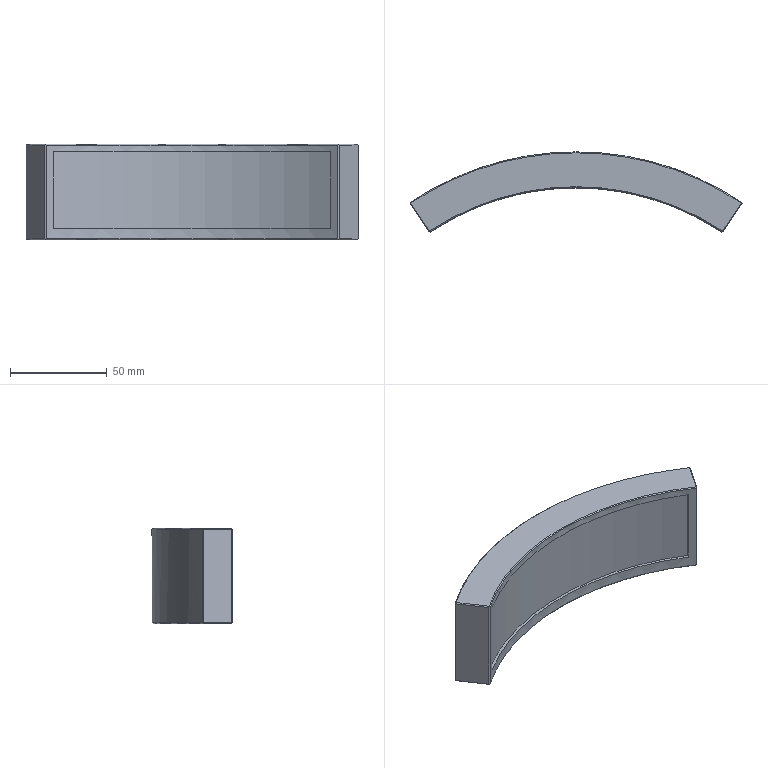Part | SolidWorks | features BaseBody 1 | 1 solid | 47 faces | box 171.672 x 41.389 x 49.5 mm | volume 148043 mm3 | plane 25 | cone 11 | cylinder 11 | commonest cylinder face diameters 2.5 x6 3.5 x2 271 x1 274 x1 308 x1
STEP:
#1=CARTESIAN_POINT('',(-85.424,127.536,49.5));
#2=VERTEX_POINT('',#1);
#3=CARTESIAN_POINT('',(0.,153.501,49.5));
#4=VERTEX_POINT('',#3);
#5=CARTESIAN_POINT('',(0.,0.,49.5));
#6=DIRECTION('',(0.,0.,-1.));
#7=DIRECTION('',(0.,1.,0.));
#8=AXIS2_PLACEMENT_3D('',#5,#6,#7);
#9=CIRCLE('',#8,153.501);
#10=EDGE_CURVE('',#2,#4,#9,.T.);
#11=ORIENTED_EDGE('',*,*,#10,.T.);
#12=CARTESIAN_POINT('',(0.,154.,49.002));
#13=VERTEX_POINT('',#12);
#14=CARTESIAN_POINT('',(0.,154.,49.002));
#15=DIRECTION('',(0.,0.7083,-0.706));
#16=VECTOR('',#15,1000.);
#17=LINE('',#14,#16);
#18=EDGE_CURVE('',#4,#13,#17,.T.);
#19=ORIENTED_EDGE('',*,*,#18,.T.);
#20=CARTESIAN_POINT('',(-85.701,127.95,49.002));
#21=VERTEX_POINT('',#20);
#22=CARTESIAN_POINT('',(0.,0.,49.002));
#23=DIRECTION('',(0.,0.,-1.));
#24=DIRECTION('',(-1.,0.,0.));
#25=AXIS2_PLACEMENT_3D('',#22,#23,#24);
#26=CIRCLE('',#25,154.);
#27=EDGE_CURVE('',#21,#13,#26,.T.);
#28=ORIENTED_EDGE('',*,*,#27,.F.);
#29=CARTESIAN_POINT('',(-85.424,127.536,49.5));
#30=DIRECTION('',(0.3941,-0.5885,0.706));
#31=VECTOR('',#30,1000.);
#32=LINE('',#29,#31);
#33=EDGE_CURVE('',#21,#2,#32,.T.);
#34=ORIENTED_EDGE('',*,*,#33,.T.);
#35=EDGE_LOOP('',(#11,#19,#28,#34));
#36=FACE_OUTER_BOUND('',#35,.T.);
#37=CARTESIAN_POINT('',(0.,0.,49.002));
#38=DIRECTION('',(0.,0.,-1.));
#39=DIRECTION('',(0.,1.,0.));
#40=AXIS2_PLACEMENT_3D('',#37,#38,#39);
#41=CONICAL_SURFACE('',#40,154.,0.787);
#42=ADVANCED_FACE('',(#36),#41,.T.);
#43=CARTESIAN_POINT('',(52.605,139.416,43.5));
#44=VERTEX_POINT('',#43);
#45=CARTESIAN_POINT('',(49.317,140.613,43.5));
#46=VERTEX_POINT('',#45);
#47=CARTESIAN_POINT('',(50.961,140.014,43.5));
#48=DIRECTION('',(0.342,0.9397,0.));
#49=DIRECTION('',(-0.9397,0.342,0.));
#50=AXIS2_PLACEMENT_3D('',#47,#48,#49);
#51=CIRCLE('',#50,1.75);
#52=EDGE_CURVE('',#44,#46,#51,.T.);
#53=ORIENTED_EDGE('',*,*,#52,.F.);
#54=CARTESIAN_POINT('',(54.312,144.105,43.5));
#55=VERTEX_POINT('',#54);
#56=CARTESIAN_POINT('',(54.316,144.114,43.5));
#57=DIRECTION('',(0.342,0.9397,0.));
#58=VECTOR('',#57,1000.);
#59=LINE('',#56,#58);
#60=EDGE_CURVE('',#44,#55,#59,.T.);
#61=ORIENTED_EDGE('',*,*,#60,.T.);
#62=CARTESIAN_POINT('',(51.023,145.302,43.5));
#63=VERTEX_POINT('',#62);
#64=CARTESIAN_POINT('',(51.023,145.302,43.5));
#65=CARTESIAN_POINT('',(51.023,145.302,43.384));
#66=CARTESIAN_POINT('',(51.034,145.298,43.271));
#67=CARTESIAN_POINT('',(51.076,145.283,43.047));
#68=CARTESIAN_POINT('',(51.108,145.272,42.936));
#69=CARTESIAN_POINT('',(51.19,145.243,42.724));
#70=CARTESIAN_POINT('',(51.241,145.225,42.624));
#71=CARTESIAN_POINT('',(51.361,145.183,42.433));
#72=CARTESIAN_POINT('',(51.431,145.158,42.343));
#73=CARTESIAN_POINT('',(51.659,145.077,42.101));
#74=CARTESIAN_POINT('',(51.843,145.012,41.971));
#75=CARTESIAN_POINT('',(52.239,144.869,41.796));
#76=CARTESIAN_POINT('',(52.456,144.791,41.75));
#77=CARTESIAN_POINT('',(52.777,144.674,41.75));
#78=CARTESIAN_POINT('',(52.886,144.634,41.761));
#79=CARTESIAN_POINT('',(53.097,144.557,41.806));
#80=CARTESIAN_POINT('',(53.199,144.519,41.839));
#81=CARTESIAN_POINT('',(53.398,144.446,41.926));
#82=CARTESIAN_POINT('',(53.494,144.41,41.981));
#83=CARTESIAN_POINT('',(53.672,144.344,42.108));
#84=CARTESIAN_POINT('',(53.755,144.314,42.18));
#85=CARTESIAN_POINT('',(53.908,144.257,42.343));
#86=CARTESIAN_POINT('',(53.976,144.231,42.432));
#87=CARTESIAN_POINT('',(54.095,144.187,42.621));
#88=CARTESIAN_POINT('',(54.146,144.167,42.723));
#89=CARTESIAN_POINT('',(54.269,144.121,43.042));
#90=CARTESIAN_POINT('',(54.312,144.105,43.269));
#91=CARTESIAN_POINT('',(54.312,144.105,43.5));
#92=B_SPLINE_CURVE_WITH_KNOTS('',3,(#64,#65,#66,#67,#68,#69,#70,#71,#72,#73,#74,#75,#76,#77,#78,#79,#80,#81,#82,#83,#84,#85,#86,#87,#88,#89,#90,#91),.UNSPECIFIED.,.F.,.F.,(4,2,2,2,2,2,2,2,2,2,2,2,2,4),(0.,0.0003419,0.0006838,0.001026,0.001368,0.002051,0.002735,0.003077,0.003419,0.003761,0.004103,0.004445,0.004786,0.00547),.UNSPECIFIED.);
#93=EDGE_CURVE('',#63,#55,#92,.T.);
#94=ORIENTED_EDGE('',*,*,#93,.F.);
#95=CARTESIAN_POINT('',(51.027,145.311,43.5));
#96=DIRECTION('',(0.342,0.9397,0.));
#97=VECTOR('',#96,1000.);
#98=LINE('',#95,#97);
#99=EDGE_CURVE('',#46,#63,#98,.T.);
#100=ORIENTED_EDGE('',*,*,#99,.F.);
#101=EDGE_LOOP('',(#53,#61,#94,#100));
#102=FACE_OUTER_BOUND('',#101,.T.);
#103=CARTESIAN_POINT('',(52.671,144.713,43.5));
#104=DIRECTION('',(0.342,0.9397,0.));
#105=DIRECTION('',(-0.9397,0.342,0.));
#106=AXIS2_PLACEMENT_3D('',#103,#104,#105);
#107=CYLINDRICAL_SURFACE('',#106,1.75);
#108=ADVANCED_FACE('',(#102),#107,.F.);
#109=CARTESIAN_POINT('',(1.25,143.5,6.));
#110=VERTEX_POINT('',#109);
#111=CARTESIAN_POINT('',(-1.25,143.5,6.));
#112=VERTEX_POINT('',#111);
#113=CARTESIAN_POINT('',(0.,143.5,6.));
#114=DIRECTION('',(0.,0.,-1.));
#115=DIRECTION('',(-1.,0.,0.));
#116=AXIS2_PLACEMENT_3D('',#113,#114,#115);
#117=CIRCLE('',#116,1.25);
#118=EDGE_CURVE('',#110,#112,#117,.T.);
#119=ORIENTED_EDGE('',*,*,#118,.F.);
#120=CARTESIAN_POINT('',(1.25,143.5,0.));
#121=VERTEX_POINT('',#120);
#122=CARTESIAN_POINT('',(1.25,143.5,0.));
#123=DIRECTION('',(0.,0.,-1.));
#124=VECTOR('',#123,1000.);
#125=LINE('',#122,#124);
#126=EDGE_CURVE('',#110,#121,#125,.T.);
#127=ORIENTED_EDGE('',*,*,#126,.T.);
#128=CARTESIAN_POINT('',(-1.25,143.5,0.));
#129=VERTEX_POINT('',#128);
#130=CARTESIAN_POINT('',(0.,143.5,0.));
#131=DIRECTION('',(0.,0.,-1.));
#132=DIRECTION('',(-1.,0.,0.));
#133=AXIS2_PLACEMENT_3D('',#130,#131,#132);
#134=CIRCLE('',#133,1.25);
#135=EDGE_CURVE('',#121,#129,#134,.T.);
#136=ORIENTED_EDGE('',*,*,#135,.T.);
#137=CARTESIAN_POINT('',(-1.25,143.5,0.));
#138=DIRECTION('',(0.,0.,-1.));
#139=VECTOR('',#138,1000.);
#140=LINE('',#137,#139);
#141=EDGE_CURVE('',#112,#129,#140,.T.);
#142=ORIENTED_EDGE('',*,*,#141,.F.);
#143=EDGE_LOOP('',(#119,#127,#136,#142));
#144=FACE_OUTER_BOUND('',#143,.T.);
#145=CARTESIAN_POINT('',(0.,143.5,0.));
#146=DIRECTION('',(0.,0.,-1.));
#147=DIRECTION('',(-1.,0.,0.));
#148=AXIS2_PLACEMENT_3D('',#145,#146,#147);
#149=CYLINDRICAL_SURFACE('',#148,1.25);
#150=ADVANCED_FACE('',(#144),#149,.F.);
#151=CARTESIAN_POINT('',(49.269,135.227,6.));
#152=VERTEX_POINT('',#151);
#153=CARTESIAN_POINT('',(48.019,133.977,6.));
#154=VERTEX_POINT('',#153);
#155=CARTESIAN_POINT('',(48.019,135.227,6.));
#156=DIRECTION('',(0.,0.,-1.));
#157=DIRECTION('',(-1.,0.,0.));
#158=AXIS2_PLACEMENT_3D('',#155,#156,#157);
#159=CIRCLE('',#158,1.25);
#160=EDGE_CURVE('',#152,#154,#159,.T.);
#161=ORIENTED_EDGE('',*,*,#160,.F.);
#162=CARTESIAN_POINT('',(49.269,135.227,0.));
#163=VERTEX_POINT('',#162);
#164=CARTESIAN_POINT('',(49.269,135.227,0.));
#165=DIRECTION('',(0.,0.,-1.));
#166=VECTOR('',#165,1000.);
#167=LINE('',#164,#166);
#168=EDGE_CURVE('',#152,#163,#167,.T.);
#169=ORIENTED_EDGE('',*,*,#168,.T.);
#170=CARTESIAN_POINT('',(46.769,135.227,0.));
#171=VERTEX_POINT('',#170);
#172=CARTESIAN_POINT('',(48.019,135.227,0.));
#173=DIRECTION('',(0.,0.,-1.));
#174=DIRECTION('',(-1.,0.,0.));
#175=AXIS2_PLACEMENT_3D('',#172,#173,#174);
#176=CIRCLE('',#175,1.25);
#177=EDGE_CURVE('',#163,#171,#176,.T.);
#178=ORIENTED_EDGE('',*,*,#177,.T.);
#179=CARTESIAN_POINT('',(46.769,135.227,6.));
#180=VERTEX_POINT('',#179);
#181=CARTESIAN_POINT('',(46.769,135.227,0.));
#182=DIRECTION('',(0.,0.,-1.));
#183=VECTOR('',#182,1000.);
#184=LINE('',#181,#183);
#185=EDGE_CURVE('',#180,#171,#184,.T.);
#186=ORIENTED_EDGE('',*,*,#185,.F.);
#187=CARTESIAN_POINT('',(48.019,135.227,6.));
#188=DIRECTION('',(0.,0.,-1.));
#189=DIRECTION('',(-1.,0.,0.));
#190=AXIS2_PLACEMENT_3D('',#187,#188,#189);
#191=CIRCLE('',#190,1.25);
#192=EDGE_CURVE('',#154,#180,#191,.T.);
#193=ORIENTED_EDGE('',*,*,#192,.F.);
#194=EDGE_LOOP('',(#161,#169,#178,#186,#193));
#195=FACE_OUTER_BOUND('',#194,.T.);
#196=CARTESIAN_POINT('',(48.019,135.227,0.));
#197=DIRECTION('',(0.,0.,-1.));
#198=DIRECTION('',(-1.,0.,0.));
#199=AXIS2_PLACEMENT_3D('',#196,#197,#198);
#200=CYLINDRICAL_SURFACE('',#199,1.25);
#201=ADVANCED_FACE('',(#195),#200,.F.);
#202=CARTESIAN_POINT('',(-46.769,135.227,6.));
#203=VERTEX_POINT('',#202);
#204=CARTESIAN_POINT('',(-49.269,135.227,6.));
#205=VERTEX_POINT('',#204);
#206=CARTESIAN_POINT('',(-48.019,135.227,6.));
#207=DIRECTION('',(0.,0.,-1.));
#208=DIRECTION('',(-1.,0.,0.));
#209=AXIS2_PLACEMENT_3D('',#206,#207,#208);
#210=CIRCLE('',#209,1.25);
#211=EDGE_CURVE('',#203,#205,#210,.T.);
#212=ORIENTED_EDGE('',*,*,#211,.F.);
#213=CARTESIAN_POINT('',(-46.769,135.227,0.));
#214=VERTEX_POINT('',#213);
#215=CARTESIAN_POINT('',(-46.769,135.227,0.));
#216=DIRECTION('',(0.,0.,-1.));
#217=VECTOR('',#216,1000.);
#218=LINE('',#215,#217);
#219=EDGE_CURVE('',#203,#214,#218,.T.);
#220=ORIENTED_EDGE('',*,*,#219,.T.);
#221=CARTESIAN_POINT('',(-49.269,135.227,0.));
#222=VERTEX_POINT('',#221);
#223=CARTESIAN_POINT('',(-48.019,135.227,0.));
#224=DIRECTION('',(0.,0.,-1.));
#225=DIRECTION('',(-1.,0.,0.));
#226=AXIS2_PLACEMENT_3D('',#223,#224,#225);
#227=CIRCLE('',#226,1.25);
#228=EDGE_CURVE('',#214,#222,#227,.T.);
#229=ORIENTED_EDGE('',*,*,#228,.T.);
#230=CARTESIAN_POINT('',(-49.269,135.227,0.));
#231=DIRECTION('',(0.,0.,-1.));
#232=VECTOR('',#231,1000.);
#233=LINE('',#230,#232);
#234=EDGE_CURVE('',#205,#222,#233,.T.);
#235=ORIENTED_EDGE('',*,*,#234,.F.);
#236=EDGE_LOOP('',(#212,#220,#229,#235));
#237=FACE_OUTER_BOUND('',#236,.T.);
#238=CARTESIAN_POINT('',(-48.019,135.227,0.));
#239=DIRECTION('',(0.,0.,-1.));
#240=DIRECTION('',(-1.,0.,0.));
#241=AXIS2_PLACEMENT_3D('',#238,#239,#240);
#242=CYLINDRICAL_SURFACE('',#241,1.25);
#243=ADVANCED_FACE('',(#237),#242,.F.);
#244=CARTESIAN_POINT('',(0.,143.5,6.751));
#245=VERTEX_POINT('',#244);
#246=CARTESIAN_POINT('',(-1.25,143.5,6.));
#247=DIRECTION('',(-0.8572,0.,-0.515));
#248=VECTOR('',#247,1000.);
#249=LINE('',#246,#248);
#250=EDGE_CURVE('',#245,#112,#249,.T.);
#251=ORIENTED_EDGE('',*,*,#250,.F.);
#252=CARTESIAN_POINT('',(1.25,143.5,6.));
#253=DIRECTION('',(0.8572,0.,-0.515));
#254=VECTOR('',#253,1000.);
#255=LINE('',#252,#254);
#256=EDGE_CURVE('',#245,#110,#255,.T.);
#257=ORIENTED_EDGE('',*,*,#256,.T.);
#258=ORIENTED_EDGE('',*,*,#118,.T.);
#259=EDGE_LOOP('',(#251,#257,#258));
#260=FACE_OUTER_BOUND('',#259,.T.);
#261=CARTESIAN_POINT('',(0.,143.5,6.));
#262=DIRECTION('',(0.,0.,-1.));
#263=DIRECTION('',(-1.,0.,0.));
#264=AXIS2_PLACEMENT_3D('',#261,#262,#263);
#265=CONICAL_SURFACE('',#264,1.25,1.03);
#266=ADVANCED_FACE('',(#260),#265,.F.);
#267=CARTESIAN_POINT('',(48.019,135.227,6.751));
#268=VERTEX_POINT('',#267);
#269=CARTESIAN_POINT('',(48.019,136.477,6.));
#270=VERTEX_POINT('',#269);
#271=CARTESIAN_POINT('',(48.019,136.477,6.));
#272=DIRECTION('',(0.,0.8572,-0.515));
#273=VECTOR('',#272,1000.);
#274=LINE('',#271,#273);
#275=EDGE_CURVE('',#268,#270,#274,.T.);
#276=ORIENTED_EDGE('',*,*,#275,.F.);
#277=CARTESIAN_POINT('',(48.019,133.977,6.));
#278=DIRECTION('',(0.,-0.8572,-0.515));
#279=VECTOR('',#278,1000.);
#280=LINE('',#277,#279);
#281=EDGE_CURVE('',#268,#154,#280,.T.);
#282=ORIENTED_EDGE('',*,*,#281,.T.);
#283=ORIENTED_EDGE('',*,*,#192,.T.);
#284=CARTESIAN_POINT('',(48.019,135.227,6.));
#285=DIRECTION('',(0.,0.,-1.));
#286=DIRECTION('',(-1.,0.,0.));
#287=AXIS2_PLACEMENT_3D('',#284,#285,#286);
#288=CIRCLE('',#287,1.25);
#289=EDGE_CURVE('',#180,#270,#288,.T.);
#290=ORIENTED_EDGE('',*,*,#289,.T.);
#291=EDGE_LOOP('',(#276,#282,#283,#290));
#292=FACE_OUTER_BOUND('',#291,.T.);
#293=CARTESIAN_POINT('',(48.019,135.227,6.));
#294=DIRECTION('',(0.,0.,-1.));
#295=DIRECTION('',(0.,1.,0.));
#296=AXIS2_PLACEMENT_3D('',#293,#294,#295);
#297=CONICAL_SURFACE('',#296,1.25,1.03);
#298=ADVANCED_FACE('',(#292),#297,.F.);
#299=CARTESIAN_POINT('',(-48.019,135.227,6.751));
#300=VERTEX_POINT('',#299);
#301=CARTESIAN_POINT('',(-49.269,135.227,6.));
#302=DIRECTION('',(-0.8572,0.,-0.515));
#303=VECTOR('',#302,1000.);
#304=LINE('',#301,#303);
#305=EDGE_CURVE('',#300,#205,#304,.T.);
#306=ORIENTED_EDGE('',*,*,#305,.F.);
#307=CARTESIAN_POINT('',(-46.769,135.227,6.));
#308=DIRECTION('',(0.8572,0.,-0.515));
#309=VECTOR('',#308,1000.);
#310=LINE('',#307,#309);
#311=EDGE_CURVE('',#300,#203,#310,.T.);
#312=ORIENTED_EDGE('',*,*,#311,.T.);
#313=ORIENTED_EDGE('',*,*,#211,.T.);
#314=EDGE_LOOP('',(#306,#312,#313));
#315=FACE_OUTER_BOUND('',#314,.T.);
#316=CARTESIAN_POINT('',(-48.019,135.227,6.));
#317=DIRECTION('',(0.,0.,-1.));
#318=DIRECTION('',(-1.,0.,0.));
#319=AXIS2_PLACEMENT_3D('',#316,#317,#318);
#320=CONICAL_SURFACE('',#319,1.25,1.03);
#321=ADVANCED_FACE('',(#315),#320,.F.);
#322=ORIENTED_EDGE('',*,*,#27,.T.);
#323=CARTESIAN_POINT('',(85.701,127.95,49.002));
#324=VERTEX_POINT('',#323);
#325=CARTESIAN_POINT('',(0.,0.,49.002));
#326=DIRECTION('',(0.,0.,-1.));
#327=DIRECTION('',(-1.,0.,0.));
#328=AXIS2_PLACEMENT_3D('',#325,#326,#327);
#329=CIRCLE('',#328,154.);
#330=EDGE_CURVE('',#13,#324,#329,.T.);
#331=ORIENTED_EDGE('',*,*,#330,.T.);
#332=CARTESIAN_POINT('',(85.701,127.95,0.4976));
#333=VERTEX_POINT('',#332);
#334=CARTESIAN_POINT('',(85.701,127.95,49.5));
#335=DIRECTION('',(0.,0.,-1.));
#336=VECTOR('',#335,1000.);
#337=LINE('',#334,#336);
#338=EDGE_CURVE('',#324,#333,#337,.T.);
#339=ORIENTED_EDGE('',*,*,#338,.T.);
#340=CARTESIAN_POINT('',(-85.701,127.95,0.4976));
#341=VERTEX_POINT('',#340);
#342=CARTESIAN_POINT('',(0.,0.,0.4976));
#343=DIRECTION('',(0.,0.,1.));
#344=DIRECTION('',(-1.,0.,0.));
#345=AXIS2_PLACEMENT_3D('',#342,#343,#344);
#346=CIRCLE('',#345,154.);
#347=EDGE_CURVE('',#333,#341,#346,.T.);
#348=ORIENTED_EDGE('',*,*,#347,.T.);
#349=CARTESIAN_POINT('',(-85.701,127.95,49.5));
#350=DIRECTION('',(0.,0.,1.));
#351=VECTOR('',#350,1000.);
#352=LINE('',#349,#351);
#353=EDGE_CURVE('',#341,#21,#352,.T.);
#354=ORIENTED_EDGE('',*,*,#353,.T.);
#355=EDGE_LOOP('',(#322,#331,#339,#348,#354));
#356=FACE_OUTER_BOUND('',#355,.T.);
#357=ORIENTED_EDGE('',*,*,#93,.T.);
#358=CARTESIAN_POINT('',(54.312,144.105,43.5));
#359=CARTESIAN_POINT('',(54.312,144.105,43.616));
#360=CARTESIAN_POINT('',(54.302,144.109,43.729));
#361=CARTESIAN_POINT('',(54.26,144.124,43.953));
#362=CARTESIAN_POINT('',(54.228,144.136,44.064));
#363=CARTESIAN_POINT('',(54.146,144.167,44.276));
#364=CARTESIAN_POINT('',(54.096,144.186,44.376));
#365=CARTESIAN_POINT('',(53.977,144.231,44.567));
#366=CARTESIAN_POINT('',(53.908,144.257,44.657));
#367=CARTESIAN_POINT('',(53.681,144.341,44.899));
#368=CARTESIAN_POINT('',(53.498,144.409,45.029));
#369=CARTESIAN_POINT('',(53.103,144.555,45.204));
#370=CARTESIAN_POINT('',(52.887,144.634,45.25));
#371=CARTESIAN_POINT('',(52.565,144.751,45.25));
#372=CARTESIAN_POINT('',(52.456,144.791,45.239));
#373=CARTESIAN_POINT('',(52.245,144.867,45.194));
#374=CARTESIAN_POINT('',(52.142,144.904,45.161));
#375=CARTESIAN_POINT('',(51.943,144.976,45.074));
#376=CARTESIAN_POINT('',(51.846,145.01,45.019));
#377=CARTESIAN_POINT('',(51.668,145.074,44.892));
#378=CARTESIAN_POINT('',(51.584,145.104,44.82));
#379=CARTESIAN_POINT('',(51.43,145.158,44.657));
#380=CARTESIAN_POINT('',(51.362,145.182,44.568));
#381=CARTESIAN_POINT('',(51.242,145.225,44.379));
#382=CARTESIAN_POINT('',(51.191,145.243,44.277));
#383=CARTESIAN_POINT('',(51.066,145.287,43.958));
#384=CARTESIAN_POINT('',(51.023,145.302,43.731));
#385=CARTESIAN_POINT('',(51.023,145.302,43.5));
#386=B_SPLINE_CURVE_WITH_KNOTS('',3,(#358,#359,#360,#361,#362,#363,#364,#365,#366,#367,#368,#369,#370,#371,#372,#373,#374,#375,#376,#377,#378,#379,#380,#381,#382,#383,#384,#385),.UNSPECIFIED.,.F.,.F.,(4,2,2,2,2,2,2,2,2,2,2,2,2,4),(0.00547,0.005812,0.006154,0.006496,0.006838,0.007522,0.008205,0.008547,0.008889,0.009231,0.009573,0.009915,0.01026,0.01094),.UNSPECIFIED.);
#387=EDGE_CURVE('',#55,#63,#386,.T.);
#388=ORIENTED_EDGE('',*,*,#387,.T.);
#389=EDGE_LOOP('',(#357,#388));
#390=FACE_BOUND('',#389,.T.);
#391=CARTESIAN_POINT('',(0.,0.,49.5));
#392=DIRECTION('',(0.,0.,-1.));
#393=DIRECTION('',(-1.,0.,0.));
#394=AXIS2_PLACEMENT_3D('',#391,#392,#393);
#395=CYLINDRICAL_SURFACE('',#394,154.);
#396=ADVANCED_FACE('',(#356,#390),#395,.T.);
#397=ORIENTED_EDGE('',*,*,#338,.F.);
#398=CARTESIAN_POINT('',(85.836,127.257,49.001));
#399=VERTEX_POINT('',#398);
#400=CARTESIAN_POINT('',(85.836,127.257,49.001));
#401=DIRECTION('',(-0.1908,0.9816,0.002296));
#402=VECTOR('',#401,1000.);
#403=LINE('',#400,#402);
#404=EDGE_CURVE('',#399,#324,#403,.T.);
#405=ORIENTED_EDGE('',*,*,#404,.F.);
#406=CARTESIAN_POINT('',(85.836,127.257,0.4992));
#407=VERTEX_POINT('',#406);
#408=CARTESIAN_POINT('',(85.836,127.257,49.5));
#409=DIRECTION('',(0.,0.,1.));
#410=VECTOR('',#409,1000.);
#411=LINE('',#408,#410);
#412=EDGE_CURVE('',#407,#399,#411,.T.);
#413=ORIENTED_EDGE('',*,*,#412,.F.);
#414=CARTESIAN_POINT('',(85.701,127.95,0.4976));
#415=DIRECTION('',(0.1908,-0.9816,0.002296));
#416=VECTOR('',#415,1000.);
#417=LINE('',#414,#416);
#418=EDGE_CURVE('',#333,#407,#417,.T.);
#419=ORIENTED_EDGE('',*,*,#418,.F.);
#420=EDGE_LOOP('',(#397,#405,#413,#419));
#421=FACE_OUTER_BOUND('',#420,.T.);
#422=CARTESIAN_POINT('',(85.701,127.95,49.5));
#423=DIRECTION('',(-0.9816,-0.1908,0.));
#424=DIRECTION('',(0.1908,-0.9816,0.));
#425=AXIS2_PLACEMENT_3D('',#422,#423,#424);
#426=PLANE('',#425);
#427=ADVANCED_FACE('',(#421),#426,.F.);
#428=ORIENTED_EDGE('',*,*,#18,.F.);
#429=CARTESIAN_POINT('',(85.424,127.536,49.5));
#430=VERTEX_POINT('',#429);
#431=CARTESIAN_POINT('',(0.,0.,49.5));
#432=DIRECTION('',(0.,0.,-1.));
#433=DIRECTION('',(0.,1.,0.));
#434=AXIS2_PLACEMENT_3D('',#431,#432,#433);
#435=CIRCLE('',#434,153.501);
#436=EDGE_CURVE('',#4,#430,#435,.T.);
#437=ORIENTED_EDGE('',*,*,#436,.T.);
#438=CARTESIAN_POINT('',(85.424,127.536,49.5));
#439=DIRECTION('',(0.3941,0.5885,-0.706));
#440=VECTOR('',#439,1000.);
#441=LINE('',#438,#440);
#442=EDGE_CURVE('',#430,#324,#441,.T.);
#443=ORIENTED_EDGE('',*,*,#442,.T.);
#444=ORIENTED_EDGE('',*,*,#330,.F.);
#445=EDGE_LOOP('',(#428,#437,#443,#444));
#446=FACE_OUTER_BOUND('',#445,.T.);
#447=CARTESIAN_POINT('',(0.,0.,49.002));
#448=DIRECTION('',(0.,0.,-1.));
#449=DIRECTION('',(0.,1.,0.));
#450=AXIS2_PLACEMENT_3D('',#447,#448,#449);
#451=CONICAL_SURFACE('',#450,154.,0.787);
#452=ADVANCED_FACE('',(#446),#451,.T.);
#453=CARTESIAN_POINT('',(-85.836,127.257,49.001));
#454=VERTEX_POINT('',#453);
#455=CARTESIAN_POINT('',(-85.836,127.257,0.4976));
#456=VERTEX_POINT('',#455);
#457=CARTESIAN_POINT('',(-85.836,127.257,49.5));
#458=DIRECTION('',(0.,0.,-1.));
#459=VECTOR('',#458,1000.);
#460=LINE('',#457,#459);
#461=EDGE_CURVE('',#454,#456,#460,.T.);
#462=ORIENTED_EDGE('',*,*,#461,.F.);
#463=CARTESIAN_POINT('',(-85.701,127.95,49.002));
#464=DIRECTION('',(-0.1908,-0.9816,-0.002296));
#465=VECTOR('',#464,1000.);
#466=LINE('',#463,#465);
#467=EDGE_CURVE('',#21,#454,#466,.T.);
#468=ORIENTED_EDGE('',*,*,#467,.F.);
#469=ORIENTED_EDGE('',*,*,#353,.F.);
#470=CARTESIAN_POINT('',(-85.836,127.257,0.4976));
#471=DIRECTION('',(0.1908,0.9816,0.));
#472=VECTOR('',#471,1000.);
#473=LINE('',#470,#472);
#474=EDGE_CURVE('',#456,#341,#473,.T.);
#475=ORIENTED_EDGE('',*,*,#474,.F.);
#476=EDGE_LOOP('',(#462,#468,#469,#475));
#477=FACE_OUTER_BOUND('',#476,.T.);
#478=CARTESIAN_POINT('',(-85.836,127.257,49.5));
#479=DIRECTION('',(0.9816,-0.1908,0.));
#480=DIRECTION('',(0.1908,0.9816,0.));
#481=AXIS2_PLACEMENT_3D('',#478,#479,#480);
#482=PLANE('',#481);
#483=ADVANCED_FACE('',(#477),#482,.F.);
#484=CARTESIAN_POINT('',(-85.422,127.536,0.));
#485=VERTEX_POINT('',#484);
#486=CARTESIAN_POINT('',(-85.422,127.536,0.));
#487=CARTESIAN_POINT('',(-85.515,127.674,0.1659));
#488=CARTESIAN_POINT('',(-85.608,127.812,0.3317));
#489=CARTESIAN_POINT('',(-85.701,127.95,0.4976));
#490=B_SPLINE_CURVE_WITH_KNOTS('',3,(#486,#487,#488,#489),.UNSPECIFIED.,.F.,.F.,(4,4),(0.,1.),.UNSPECIFIED.);
#491=EDGE_CURVE('',#485,#341,#490,.T.);
#492=ORIENTED_EDGE('',*,*,#491,.T.);
#493=ORIENTED_EDGE('',*,*,#347,.F.);
#494=CARTESIAN_POINT('',(85.424,127.536,0.));
#495=VERTEX_POINT('',#494);
#496=CARTESIAN_POINT('',(85.701,127.95,0.4976));
#497=DIRECTION('',(-0.3941,-0.5885,-0.706));
#498=VECTOR('',#497,1000.);
#499=LINE('',#496,#498);
#500=EDGE_CURVE('',#333,#495,#499,.T.);
#501=ORIENTED_EDGE('',*,*,#500,.T.);
#502=CARTESIAN_POINT('',(0.,0.,0.));
#503=DIRECTION('',(0.,0.,1.));
#504=DIRECTION('',(1.,0.,0.));
#505=AXIS2_PLACEMENT_3D('',#502,#503,#504);
#506=CIRCLE('',#505,153.501);
#507=EDGE_CURVE('',#495,#485,#506,.T.);
#508=ORIENTED_EDGE('',*,*,#507,.T.);
#509=EDGE_LOOP('',(#492,#493,#501,#508));
#510=FACE_OUTER_BOUND('',#509,.T.);
#511=CARTESIAN_POINT('',(0.,0.,0.4976));
#512=DIRECTION('',(0.,0.,1.));
#513=DIRECTION('',(1.,0.,0.));
#514=AXIS2_PLACEMENT_3D('',#511,#512,#513);
#515=CONICAL_SURFACE('',#514,154.,0.787);
#516=ADVANCED_FACE('',(#510),#515,.T.);
#517=ORIENTED_EDGE('',*,*,#60,.F.);
#518=CARTESIAN_POINT('',(50.961,140.014,43.5));
#519=DIRECTION('',(0.342,0.9397,0.));
#520=DIRECTION('',(-0.9397,0.342,0.));
#521=AXIS2_PLACEMENT_3D('',#518,#519,#520);
#522=CIRCLE('',#521,1.75);
#523=EDGE_CURVE('',#46,#44,#522,.T.);
#524=ORIENTED_EDGE('',*,*,#523,.F.);
#525=ORIENTED_EDGE('',*,*,#99,.T.);
#526=ORIENTED_EDGE('',*,*,#387,.F.);
#527=EDGE_LOOP('',(#517,#524,#525,#526));
#528=FACE_OUTER_BOUND('',#527,.T.);
#529=CARTESIAN_POINT('',(52.671,144.713,43.5));
#530=DIRECTION('',(0.342,0.9397,0.));
#531=DIRECTION('',(-0.9397,0.342,0.));
#532=AXIS2_PLACEMENT_3D('',#529,#530,#531);
#533=CYLINDRICAL_SURFACE('',#532,1.75);
#534=ADVANCED_FACE('',(#528),#533,.F.);
#535=CARTESIAN_POINT('',(85.836,127.257,0.4992));
#536=DIRECTION('',(-0.5853,0.3948,-0.7083));
#537=VECTOR('',#536,1000.);
#538=LINE('',#535,#537);
#539=EDGE_CURVE('',#407,#495,#538,.T.);
#540=ORIENTED_EDGE('',*,*,#539,.T.);
#541=ORIENTED_EDGE('',*,*,#500,.F.);
#542=ORIENTED_EDGE('',*,*,#418,.T.);
#543=EDGE_LOOP('',(#540,#541,#542));
#544=FACE_OUTER_BOUND('',#543,.T.);
#545=CARTESIAN_POINT('',(85.424,127.536,0.));
#546=DIRECTION('',(0.8022,0.1546,-0.5767));
#547=DIRECTION('',(-0.5837,0.,-0.8119));
#548=AXIS2_PLACEMENT_3D('',#545,#546,#547);
#549=PLANE('',#548);
#550=ADVANCED_FACE('',(#544),#549,.T.);
#551=ORIENTED_EDGE('',*,*,#404,.T.);
#552=ORIENTED_EDGE('',*,*,#442,.F.);
#553=CARTESIAN_POINT('',(85.836,127.257,49.001));
#554=DIRECTION('',(-0.5853,0.3948,0.7083));
#555=VECTOR('',#554,1000.);
#556=LINE('',#553,#555);
#557=EDGE_CURVE('',#399,#430,#556,.T.);
#558=ORIENTED_EDGE('',*,*,#557,.F.);
#559=EDGE_LOOP('',(#551,#552,#558));
#560=FACE_OUTER_BOUND('',#559,.T.);
#561=CARTESIAN_POINT('',(85.424,127.536,49.5));
#562=DIRECTION('',(0.8022,0.1546,0.5767));
#563=DIRECTION('',(0.5837,0.,-0.8119));
#564=AXIS2_PLACEMENT_3D('',#561,#562,#563);
#565=PLANE('',#564);
#566=ADVANCED_FACE('',(#560),#565,.T.);
#567=CARTESIAN_POINT('',(76.049,112.748,0.4992));
#568=VERTEX_POINT('',#567);
#569=CARTESIAN_POINT('',(76.049,112.748,49.001));
#570=VERTEX_POINT('',#569);
#571=CARTESIAN_POINT('',(76.049,112.748,49.5));
#572=DIRECTION('',(0.,0.,1.));
#573=VECTOR('',#572,1000.);
#574=LINE('',#571,#573);
#575=EDGE_CURVE('',#568,#570,#574,.T.);
#576=ORIENTED_EDGE('',*,*,#575,.F.);
#577=CARTESIAN_POINT('',(75.771,112.335,0.4992));
#578=DIRECTION('',(-0.5592,-0.829,0.));
#579=VECTOR('',#578,1000.);
#580=LINE('',#577,#579);
#581=EDGE_CURVE('',#407,#568,#580,.T.);
#582=ORIENTED_EDGE('',*,*,#581,.F.);
#583=ORIENTED_EDGE('',*,*,#412,.T.);
#584=CARTESIAN_POINT('',(75.771,112.335,49.001));
#585=DIRECTION('',(0.5592,0.829,0.));
#586=VECTOR('',#585,1000.);
#587=LINE('',#584,#586);
#588=EDGE_CURVE('',#570,#399,#587,.T.);
#589=ORIENTED_EDGE('',*,*,#588,.F.);
#590=EDGE_LOOP('',(#576,#582,#583,#589));
#591=FACE_OUTER_BOUND('',#590,.T.);
#592=CARTESIAN_POINT('',(75.771,112.335,49.5));
#593=DIRECTION('',(-0.829,0.5592,0.));
#594=DIRECTION('',(-0.5592,-0.829,0.));
#595=AXIS2_PLACEMENT_3D('',#592,#593,#594);
#596=PLANE('',#595);
#597=ADVANCED_FACE('',(#591),#596,.F.);
#598=CARTESIAN_POINT('',(-75.636,113.025,49.5));
#599=VERTEX_POINT('',#598);
#600=CARTESIAN_POINT('',(75.636,113.025,49.5));
#601=VERTEX_POINT('',#600);
#602=CARTESIAN_POINT('',(0.,0.,49.5));
#603=DIRECTION('',(0.,0.,-1.));
#604=DIRECTION('',(0.,-1.,0.));
#605=AXIS2_PLACEMENT_3D('',#602,#603,#604);
#606=CIRCLE('',#605,135.998);
#607=EDGE_CURVE('',#599,#601,#606,.T.);
#608=ORIENTED_EDGE('',*,*,#607,.T.);
#609=CARTESIAN_POINT('',(75.636,113.025,49.5));
#610=DIRECTION('',(0.5592,0.829,0.));
#611=VECTOR('',#610,1000.);
#612=LINE('',#609,#611);
#613=EDGE_CURVE('',#601,#430,#612,.T.);
#614=ORIENTED_EDGE('',*,*,#613,.T.);
#615=ORIENTED_EDGE('',*,*,#436,.F.);
#616=ORIENTED_EDGE('',*,*,#10,.F.);
#617=CARTESIAN_POINT('',(-85.424,127.536,49.5));
#618=DIRECTION('',(0.5592,-0.829,0.));
#619=VECTOR('',#618,1000.);
#620=LINE('',#617,#619);
#621=EDGE_CURVE('',#2,#599,#620,.T.);
#622=ORIENTED_EDGE('',*,*,#621,.T.);
#623=EDGE_LOOP('',(#608,#614,#615,#616,#622));
#624=FACE_OUTER_BOUND('',#623,.T.);
#625=CARTESIAN_POINT('',(0.,0.,49.5));
#626=DIRECTION('',(0.,0.,1.));
#627=DIRECTION('',(1.,0.,0.));
#628=AXIS2_PLACEMENT_3D('',#625,#626,#627);
#629=PLANE('',#628);
#630=ADVANCED_FACE('',(#624),#629,.T.);
#631=ORIENTED_EDGE('',*,*,#467,.T.);
#632=CARTESIAN_POINT('',(-85.836,127.257,49.001));
#633=DIRECTION('',(0.5853,0.3948,0.7083));
#634=VECTOR('',#633,1000.);
#635=LINE('',#632,#634);
#636=EDGE_CURVE('',#454,#2,#635,.T.);
#637=ORIENTED_EDGE('',*,*,#636,.T.);
#638=ORIENTED_EDGE('',*,*,#33,.F.);
#639=EDGE_LOOP('',(#631,#637,#638));
#640=FACE_OUTER_BOUND('',#639,.T.);
#641=CARTESIAN_POINT('',(-85.836,127.257,49.001));
#642=DIRECTION('',(-0.8022,0.1546,0.5767));
#643=DIRECTION('',(0.5837,0.,0.8119));
#644=AXIS2_PLACEMENT_3D('',#641,#642,#643);
#645=PLANE('',#644);
#646=ADVANCED_FACE('',(#640),#645,.T.);
#647=CARTESIAN_POINT('',(-85.422,127.536,0.));
#648=DIRECTION('',(-0.5872,-0.396,0.706));
#649=VECTOR('',#648,1000.);
#650=LINE('',#647,#649);
#651=EDGE_CURVE('',#485,#456,#650,.T.);
#652=ORIENTED_EDGE('',*,*,#651,.T.);
#653=ORIENTED_EDGE('',*,*,#474,.T.);
#654=ORIENTED_EDGE('',*,*,#491,.F.);
#655=EDGE_LOOP('',(#652,#653,#654));
#656=FACE_OUTER_BOUND('',#655,.T.);
#657=CARTESIAN_POINT('',(-85.836,127.257,0.4976));
#658=DIRECTION('',(-0.8006,0.1556,-0.5786));
#659=DIRECTION('',(-0.5857,0.,0.8105));
#660=AXIS2_PLACEMENT_3D('',#657,#658,#659);
#661=PLANE('',#660);
#662=ADVANCED_FACE('',(#656),#661,.T.);
#663=CARTESIAN_POINT('',(-76.049,112.748,49.001));
#664=VERTEX_POINT('',#663);
#665=CARTESIAN_POINT('',(-75.771,112.335,49.001));
#666=DIRECTION('',(0.5592,-0.829,0.));
#667=VECTOR('',#666,1000.);
#668=LINE('',#665,#667);
#669=EDGE_CURVE('',#454,#664,#668,.T.);
#670=ORIENTED_EDGE('',*,*,#669,.F.);
#671=ORIENTED_EDGE('',*,*,#461,.T.);
#672=CARTESIAN_POINT('',(-76.049,112.748,0.4976));
#673=VERTEX_POINT('',#672);
#674=CARTESIAN_POINT('',(-75.771,112.335,0.4976));
#675=DIRECTION('',(-0.5592,0.829,0.));
#676=VECTOR('',#675,1000.);
#677=LINE('',#674,#676);
#678=EDGE_CURVE('',#673,#456,#677,.T.);
#679=ORIENTED_EDGE('',*,*,#678,.F.);
#680=CARTESIAN_POINT('',(-76.049,112.748,49.5));
#681=DIRECTION('',(0.,0.,-1.));
#682=VECTOR('',#681,1000.);
#683=LINE('',#680,#682);
#684=EDGE_CURVE('',#664,#673,#683,.T.);
#685=ORIENTED_EDGE('',*,*,#684,.F.);
#686=EDGE_LOOP('',(#670,#671,#679,#685));
#687=FACE_OUTER_BOUND('',#686,.T.);
#688=CARTESIAN_POINT('',(-75.771,112.335,49.5));
#689=DIRECTION('',(0.829,0.5592,0.));
#690=DIRECTION('',(-0.5592,0.829,0.));
#691=AXIS2_PLACEMENT_3D('',#688,#689,#690);
#692=PLANE('',#691);
#693=ADVANCED_FACE('',(#687),#692,.F.);
#694=CARTESIAN_POINT('',(0.,143.5,0.));
#695=DIRECTION('',(0.,0.,-1.));
#696=DIRECTION('',(-1.,0.,0.));
#697=AXIS2_PLACEMENT_3D('',#694,#695,#696);
#698=CIRCLE('',#697,1.25);
#699=EDGE_CURVE('',#129,#121,#698,.T.);
#700=ORIENTED_EDGE('',*,*,#699,.F.);
#701=ORIENTED_EDGE('',*,*,#135,.F.);
#702=EDGE_LOOP('',(#700,#701));
#703=FACE_BOUND('',#702,.T.);
#704=CARTESIAN_POINT('',(48.019,135.227,0.));
#705=DIRECTION('',(0.,0.,-1.));
#706=DIRECTION('',(-1.,0.,0.));
#707=AXIS2_PLACEMENT_3D('',#704,#705,#706);
#708=CIRCLE('',#707,1.25);
#709=EDGE_CURVE('',#171,#163,#708,.T.);
#710=ORIENTED_EDGE('',*,*,#709,.F.);
#711=ORIENTED_EDGE('',*,*,#177,.F.);
#712=EDGE_LOOP('',(#710,#711));
#713=FACE_BOUND('',#712,.T.);
#714=CARTESIAN_POINT('',(-48.019,135.227,0.));
#715=DIRECTION('',(0.,0.,-1.));
#716=DIRECTION('',(-1.,0.,0.));
#717=AXIS2_PLACEMENT_3D('',#714,#715,#716);
#718=CIRCLE('',#717,1.25);
#719=EDGE_CURVE('',#222,#214,#718,.T.);
#720=ORIENTED_EDGE('',*,*,#719,.F.);
#721=ORIENTED_EDGE('',*,*,#228,.F.);
#722=EDGE_LOOP('',(#720,#721));
#723=FACE_BOUND('',#722,.T.);
#724=CARTESIAN_POINT('',(-75.635,113.027,0.));
#725=VERTEX_POINT('',#724);
#726=CARTESIAN_POINT('',(-85.422,127.536,0.));
#727=DIRECTION('',(0.5592,-0.829,0.));
#728=VECTOR('',#727,1000.);
#729=LINE('',#726,#728);
#730=EDGE_CURVE('',#485,#725,#729,.T.);
#731=ORIENTED_EDGE('',*,*,#730,.F.);
#732=ORIENTED_EDGE('',*,*,#507,.F.);
#733=CARTESIAN_POINT('',(75.637,113.026,0.));
#734=VERTEX_POINT('',#733);
#735=CARTESIAN_POINT('',(75.637,113.026,0.));
#736=DIRECTION('',(0.5592,0.829,0.));
#737=VECTOR('',#736,1000.);
#738=LINE('',#735,#737);
#739=EDGE_CURVE('',#734,#495,#738,.T.);
#740=ORIENTED_EDGE('',*,*,#739,.F.);
#741=CARTESIAN_POINT('',(0.,0.,0.));
#742=DIRECTION('',(0.,0.,-1.));
#743=DIRECTION('',(-1.,0.,0.));
#744=AXIS2_PLACEMENT_3D('',#741,#742,#743);
#745=CIRCLE('',#744,135.999);
#746=EDGE_CURVE('',#725,#734,#745,.T.);
#747=ORIENTED_EDGE('',*,*,#746,.F.);
#748=EDGE_LOOP('',(#731,#732,#740,#747));
#749=FACE_OUTER_BOUND('',#748,.T.);
#750=CARTESIAN_POINT('',(0.,0.,0.));
#751=DIRECTION('',(0.,0.,1.));
#752=DIRECTION('',(1.,0.,0.));
#753=AXIS2_PLACEMENT_3D('',#750,#751,#752);
#754=PLANE('',#753);
#755=ADVANCED_FACE('',(#703,#713,#723,#749),#754,.F.);
#756=ORIENTED_EDGE('',*,*,#523,.T.);
#757=ORIENTED_EDGE('',*,*,#52,.T.);
#758=EDGE_LOOP('',(#756,#757));
#759=FACE_OUTER_BOUND('',#758,.T.);
#760=CARTESIAN_POINT('',(50.961,140.014,43.5));
#761=DIRECTION('',(-0.342,-0.9397,0.));
#762=DIRECTION('',(0.9397,-0.342,0.));
#763=AXIS2_PLACEMENT_3D('',#760,#761,#762);
#764=PLANE('',#763);
#765=ADVANCED_FACE('',(#759),#764,.F.);
#766=ORIENTED_EDGE('',*,*,#557,.T.);
#767=ORIENTED_EDGE('',*,*,#613,.F.);
#768=CARTESIAN_POINT('',(75.636,113.025,49.5));
#769=DIRECTION('',(0.5865,-0.3929,-0.7083));
#770=VECTOR('',#769,1000.);
#771=LINE('',#768,#770);
#772=EDGE_CURVE('',#601,#570,#771,.T.);
#773=ORIENTED_EDGE('',*,*,#772,.T.);
#774=ORIENTED_EDGE('',*,*,#588,.T.);
#775=EDGE_LOOP('',(#766,#767,#773,#774));
#776=FACE_OUTER_BOUND('',#775,.T.);
#777=CARTESIAN_POINT('',(-0.4125,0.2782,49.5));
#778=DIRECTION('',(0.5872,-0.3961,0.706));
#779=DIRECTION('',(0.7688,0.,-0.6395));
#780=AXIS2_PLACEMENT_3D('',#777,#778,#779);
#781=PLANE('',#780);
#782=ADVANCED_FACE('',(#776),#781,.T.);
#783=ORIENTED_EDGE('',*,*,#575,.T.);
#784=CARTESIAN_POINT('',(75.359,112.611,49.001));
#785=VERTEX_POINT('',#784);
#786=CARTESIAN_POINT('',(76.049,112.748,49.001));
#787=DIRECTION('',(0.981,0.1942,0.));
#788=VECTOR('',#787,1000.);
#789=LINE('',#786,#788);
#790=EDGE_CURVE('',#785,#570,#789,.T.);
#791=ORIENTED_EDGE('',*,*,#790,.F.);
#792=CARTESIAN_POINT('',(75.359,112.611,0.4976));
#793=VERTEX_POINT('',#792);
#794=CARTESIAN_POINT('',(75.359,112.611,49.5));
#795=DIRECTION('',(0.,0.,1.));
#796=VECTOR('',#795,1000.);
#797=LINE('',#794,#796);
#798=EDGE_CURVE('',#793,#785,#797,.T.);
#799=ORIENTED_EDGE('',*,*,#798,.F.);
#800=CARTESIAN_POINT('',(76.049,112.748,0.4992));
#801=DIRECTION('',(-0.981,-0.1942,-0.002304));
#802=VECTOR('',#801,1000.);
#803=LINE('',#800,#802);
#804=EDGE_CURVE('',#568,#793,#803,.T.);
#805=ORIENTED_EDGE('',*,*,#804,.F.);
#806=EDGE_LOOP('',(#783,#791,#799,#805));
#807=FACE_OUTER_BOUND('',#806,.T.);
#808=CARTESIAN_POINT('',(76.049,112.748,49.5));
#809=DIRECTION('',(-0.1942,0.981,0.));
#810=DIRECTION('',(-0.981,-0.1942,0.));
#811=AXIS2_PLACEMENT_3D('',#808,#809,#810);
#812=PLANE('',#811);
#813=ADVANCED_FACE('',(#807),#812,.F.);
#814=ORIENTED_EDGE('',*,*,#581,.T.);
#815=CARTESIAN_POINT('',(75.637,113.026,0.));
#816=DIRECTION('',(0.5853,-0.3948,0.7083));
#817=VECTOR('',#816,1000.);
#818=LINE('',#815,#817);
#819=EDGE_CURVE('',#734,#568,#818,.T.);
#820=ORIENTED_EDGE('',*,*,#819,.F.);
#821=ORIENTED_EDGE('',*,*,#739,.T.);
#822=ORIENTED_EDGE('',*,*,#539,.F.);
#823=EDGE_LOOP('',(#814,#820,#821,#822));
#824=FACE_OUTER_BOUND('',#823,.T.);
#825=CARTESIAN_POINT('',(75.771,112.335,0.4992));
#826=DIRECTION('',(-0.5872,0.3961,0.706));
#827=DIRECTION('',(0.7688,0.,0.6395));
#828=AXIS2_PLACEMENT_3D('',#825,#826,#827);
#829=PLANE('',#828);
#830=ADVANCED_FACE('',(#824),#829,.F.);
#831=ORIENTED_EDGE('',*,*,#607,.F.);
#832=CARTESIAN_POINT('',(-75.359,112.611,49.001));
#833=VERTEX_POINT('',#832);
#834=CARTESIAN_POINT('',(-75.359,112.611,49.001));
#835=CARTESIAN_POINT('',(-75.451,112.749,49.167));
#836=CARTESIAN_POINT('',(-75.544,112.887,49.334));
#837=CARTESIAN_POINT('',(-75.636,113.025,49.5));
#838=B_SPLINE_CURVE_WITH_KNOTS('',3,(#834,#835,#836,#837),.UNSPECIFIED.,.F.,.F.,(4,4),(0.,1.),.UNSPECIFIED.);
#839=EDGE_CURVE('',#833,#599,#838,.T.);
#840=ORIENTED_EDGE('',*,*,#839,.F.);
#841=CARTESIAN_POINT('',(0.,0.,49.001));
#842=DIRECTION('',(0.,0.,1.));
#843=DIRECTION('',(1.,0.,0.));
#844=AXIS2_PLACEMENT_3D('',#841,#842,#843);
#845=CIRCLE('',#844,135.5);
#846=EDGE_CURVE('',#785,#833,#845,.T.);
#847=ORIENTED_EDGE('',*,*,#846,.F.);
#848=CARTESIAN_POINT('',(75.636,113.025,49.5));
#849=CARTESIAN_POINT('',(75.544,112.887,49.334));
#850=CARTESIAN_POINT('',(75.451,112.749,49.167));
#851=CARTESIAN_POINT('',(75.359,112.611,49.001));
#852=B_SPLINE_CURVE_WITH_KNOTS('',3,(#848,#849,#850,#851),.UNSPECIFIED.,.F.,.F.,(4,4),(0.,1.),.UNSPECIFIED.);
#853=EDGE_CURVE('',#601,#785,#852,.T.);
#854=ORIENTED_EDGE('',*,*,#853,.F.);
#855=EDGE_LOOP('',(#831,#840,#847,#854));
#856=FACE_OUTER_BOUND('',#855,.T.);
#857=CARTESIAN_POINT('',(0.,0.,49.5));
#858=DIRECTION('',(0.,0.,1.));
#859=DIRECTION('',(0.,-1.,0.));
#860=AXIS2_PLACEMENT_3D('',#857,#858,#859);
#861=CONICAL_SURFACE('',#860,135.998,0.7838);
#862=ADVANCED_FACE('',(#856),#861,.F.);
#863=CARTESIAN_POINT('',(-76.049,112.748,49.001));
#864=DIRECTION('',(0.5865,0.3929,0.7083));
#865=VECTOR('',#864,1000.);
#866=LINE('',#863,#865);
#867=EDGE_CURVE('',#664,#599,#866,.T.);
#868=ORIENTED_EDGE('',*,*,#867,.T.);
#869=ORIENTED_EDGE('',*,*,#621,.F.);
#870=ORIENTED_EDGE('',*,*,#636,.F.);
#871=ORIENTED_EDGE('',*,*,#669,.T.);
#872=EDGE_LOOP('',(#868,#869,#870,#871));
#873=FACE_OUTER_BOUND('',#872,.T.);
#874=CARTESIAN_POINT('',(0.4125,0.2782,49.5));
#875=DIRECTION('',(-0.5872,-0.3961,0.706));
#876=DIRECTION('',(0.7688,0.,0.6395));
#877=AXIS2_PLACEMENT_3D('',#874,#875,#876);
#878=PLANE('',#877);
#879=ADVANCED_FACE('',(#873),#878,.T.);
#880=CARTESIAN_POINT('',(-75.359,112.611,0.4976));
#881=VERTEX_POINT('',#880);
#882=CARTESIAN_POINT('',(-75.359,112.611,49.5));
#883=DIRECTION('',(0.,0.,-1.));
#884=VECTOR('',#883,1000.);
#885=LINE('',#882,#884);
#886=EDGE_CURVE('',#833,#881,#885,.T.);
#887=ORIENTED_EDGE('',*,*,#886,.F.);
#888=CARTESIAN_POINT('',(-75.359,112.611,49.001));
#889=DIRECTION('',(0.981,-0.1942,0.));
#890=VECTOR('',#889,1000.);
#891=LINE('',#888,#890);
#892=EDGE_CURVE('',#664,#833,#891,.T.);
#893=ORIENTED_EDGE('',*,*,#892,.F.);
#894=ORIENTED_EDGE('',*,*,#684,.T.);
#895=CARTESIAN_POINT('',(-75.359,112.611,0.4976));
#896=DIRECTION('',(-0.981,0.1942,0.));
#897=VECTOR('',#896,1000.);
#898=LINE('',#895,#897);
#899=EDGE_CURVE('',#881,#673,#898,.T.);
#900=ORIENTED_EDGE('',*,*,#899,.F.);
#901=EDGE_LOOP('',(#887,#893,#894,#900));
#902=FACE_OUTER_BOUND('',#901,.T.);
#903=CARTESIAN_POINT('',(-75.359,112.611,49.5));
#904=DIRECTION('',(0.1942,0.981,0.));
#905=DIRECTION('',(-0.981,0.1942,0.));
#906=AXIS2_PLACEMENT_3D('',#903,#904,#905);
#907=PLANE('',#906);
#908=ADVANCED_FACE('',(#902),#907,.F.);
#909=ORIENTED_EDGE('',*,*,#730,.T.);
#910=CARTESIAN_POINT('',(-76.049,112.748,0.4976));
#911=DIRECTION('',(0.5872,0.396,-0.706));
#912=VECTOR('',#911,1000.);
#913=LINE('',#910,#912);
#914=EDGE_CURVE('',#673,#725,#913,.T.);
#915=ORIENTED_EDGE('',*,*,#914,.F.);
#916=ORIENTED_EDGE('',*,*,#678,.T.);
#917=ORIENTED_EDGE('',*,*,#651,.F.);
#918=EDGE_LOOP('',(#909,#915,#916,#917));
#919=FACE_OUTER_BOUND('',#918,.T.);
#920=CARTESIAN_POINT('',(-75.771,112.335,0.4976));
#921=DIRECTION('',(0.5853,0.3948,0.7083));
#922=DIRECTION('',(0.7709,0.,-0.637));
#923=AXIS2_PLACEMENT_3D('',#920,#921,#922);
#924=PLANE('',#923);
#925=ADVANCED_FACE('',(#919),#924,.F.);
#926=ORIENTED_EDGE('',*,*,#126,.F.);
#927=CARTESIAN_POINT('',(0.,143.5,6.));
#928=DIRECTION('',(0.,0.,-1.));
#929=DIRECTION('',(-1.,0.,0.));
#930=AXIS2_PLACEMENT_3D('',#927,#928,#929);
#931=CIRCLE('',#930,1.25);
#932=EDGE_CURVE('',#112,#110,#931,.T.);
#933=ORIENTED_EDGE('',*,*,#932,.F.);
#934=ORIENTED_EDGE('',*,*,#141,.T.);
#935=ORIENTED_EDGE('',*,*,#699,.T.);
#936=EDGE_LOOP('',(#926,#933,#934,#935));
#937=FACE_OUTER_BOUND('',#936,.T.);
#938=CARTESIAN_POINT('',(0.,143.5,0.));
#939=DIRECTION('',(0.,0.,-1.));
#940=DIRECTION('',(-1.,0.,0.));
#941=AXIS2_PLACEMENT_3D('',#938,#939,#940);
#942=CYLINDRICAL_SURFACE('',#941,1.25);
#943=ADVANCED_FACE('',(#937),#942,.F.);
#944=ORIENTED_EDGE('',*,*,#168,.F.);
#945=CARTESIAN_POINT('',(48.019,135.227,6.));
#946=DIRECTION('',(0.,0.,-1.));
#947=DIRECTION('',(-1.,0.,0.));
#948=AXIS2_PLACEMENT_3D('',#945,#946,#947);
#949=CIRCLE('',#948,1.25);
#950=EDGE_CURVE('',#270,#152,#949,.T.);
#951=ORIENTED_EDGE('',*,*,#950,.F.);
#952=ORIENTED_EDGE('',*,*,#289,.F.);
#953=ORIENTED_EDGE('',*,*,#185,.T.);
#954=ORIENTED_EDGE('',*,*,#709,.T.);
#955=EDGE_LOOP('',(#944,#951,#952,#953,#954));
#956=FACE_OUTER_BOUND('',#955,.T.);
#957=CARTESIAN_POINT('',(48.019,135.227,0.));
#958=DIRECTION('',(0.,0.,-1.));
#959=DIRECTION('',(-1.,0.,0.));
#960=AXIS2_PLACEMENT_3D('',#957,#958,#959);
#961=CYLINDRICAL_SURFACE('',#960,1.25);
#962=ADVANCED_FACE('',(#956),#961,.F.);
#963=ORIENTED_EDGE('',*,*,#219,.F.);
#964=CARTESIAN_POINT('',(-48.019,135.227,6.));
#965=DIRECTION('',(0.,0.,-1.));
#966=DIRECTION('',(-1.,0.,0.));
#967=AXIS2_PLACEMENT_3D('',#964,#965,#966);
#968=CIRCLE('',#967,1.25);
#969=EDGE_CURVE('',#205,#203,#968,.T.);
#970=ORIENTED_EDGE('',*,*,#969,.F.);
#971=ORIENTED_EDGE('',*,*,#234,.T.);
#972=ORIENTED_EDGE('',*,*,#719,.T.);
#973=EDGE_LOOP('',(#963,#970,#971,#972));
#974=FACE_OUTER_BOUND('',#973,.T.);
#975=CARTESIAN_POINT('',(-48.019,135.227,0.));
#976=DIRECTION('',(0.,0.,-1.));
#977=DIRECTION('',(-1.,0.,0.));
#978=AXIS2_PLACEMENT_3D('',#975,#976,#977);
#979=CYLINDRICAL_SURFACE('',#978,1.25);
#980=ADVANCED_FACE('',(#974),#979,.F.);
#981=CARTESIAN_POINT('',(0.,0.,0.4976));
#982=DIRECTION('',(0.,0.,-1.));
#983=DIRECTION('',(-1.,0.,0.));
#984=AXIS2_PLACEMENT_3D('',#981,#982,#983);
#985=CIRCLE('',#984,135.5);
#986=EDGE_CURVE('',#881,#793,#985,.T.);
#987=ORIENTED_EDGE('',*,*,#986,.F.);
#988=CARTESIAN_POINT('',(-75.635,113.027,0.));
#989=CARTESIAN_POINT('',(-75.543,112.888,0.1659));
#990=CARTESIAN_POINT('',(-75.451,112.75,0.3317));
#991=CARTESIAN_POINT('',(-75.359,112.611,0.4976));
#992=B_SPLINE_CURVE_WITH_KNOTS('',3,(#988,#989,#990,#991),.UNSPECIFIED.,.F.,.F.,(4,4),(0.,1.),.UNSPECIFIED.);
#993=EDGE_CURVE('',#725,#881,#992,.T.);
#994=ORIENTED_EDGE('',*,*,#993,.F.);
#995=ORIENTED_EDGE('',*,*,#746,.T.);
#996=CARTESIAN_POINT('',(75.359,112.611,0.4976));
#997=DIRECTION('',(0.3939,0.5886,-0.706));
#998=VECTOR('',#997,1000.);
#999=LINE('',#996,#998);
#1000=EDGE_CURVE('',#793,#734,#999,.T.);
#1001=ORIENTED_EDGE('',*,*,#1000,.F.);
#1002=EDGE_LOOP('',(#987,#994,#995,#1001));
#1003=FACE_OUTER_BOUND('',#1002,.T.);
#1004=CARTESIAN_POINT('',(0.,0.,0.));
#1005=DIRECTION('',(0.,0.,-1.));
#1006=DIRECTION('',(-1.,0.,0.));
#1007=AXIS2_PLACEMENT_3D('',#1004,#1005,#1006);
#1008=CONICAL_SURFACE('',#1007,135.999,0.787);
#1009=ADVANCED_FACE('',(#1003),#1008,.F.);
#1010=ORIENTED_EDGE('',*,*,#772,.F.);
#1011=ORIENTED_EDGE('',*,*,#853,.T.);
#1012=ORIENTED_EDGE('',*,*,#790,.T.);
#1013=EDGE_LOOP('',(#1010,#1011,#1012));
#1014=FACE_OUTER_BOUND('',#1013,.T.);
#1015=CARTESIAN_POINT('',(75.636,113.025,49.5));
#1016=DIRECTION('',(0.1587,-0.8018,0.5762));
#1017=DIRECTION('',(0.,-0.5836,-0.8121));
#1018=AXIS2_PLACEMENT_3D('',#1015,#1016,#1017);
#1019=PLANE('',#1018);
#1020=ADVANCED_FACE('',(#1014),#1019,.T.);
#1021=ORIENTED_EDGE('',*,*,#819,.T.);
#1022=ORIENTED_EDGE('',*,*,#804,.T.);
#1023=ORIENTED_EDGE('',*,*,#1000,.T.);
#1024=EDGE_LOOP('',(#1021,#1022,#1023));
#1025=FACE_OUTER_BOUND('',#1024,.T.);
#1026=CARTESIAN_POINT('',(75.359,112.611,0.4976));
#1027=DIRECTION('',(0.1598,-0.8002,-0.578));
#1028=DIRECTION('',(0.,0.5856,-0.8106));
#1029=AXIS2_PLACEMENT_3D('',#1026,#1027,#1028);
#1030=PLANE('',#1029);
#1031=ADVANCED_FACE('',(#1025),#1030,.T.);
#1032=CARTESIAN_POINT('',(71.804,114.911,6.));
#1033=VERTEX_POINT('',#1032);
#1034=CARTESIAN_POINT('',(71.804,114.911,45.5));
#1035=VERTEX_POINT('',#1034);
#1036=CARTESIAN_POINT('',(71.804,114.911,49.5));
#1037=DIRECTION('',(0.,0.,1.));
#1038=VECTOR('',#1037,1000.);
#1039=LINE('',#1036,#1038);
#1040=EDGE_CURVE('',#1033,#1035,#1039,.T.);
#1041=ORIENTED_EDGE('',*,*,#1040,.F.);
#1042=CARTESIAN_POINT('',(-71.804,114.911,6.));
#1043=VERTEX_POINT('',#1042);
#1044=CARTESIAN_POINT('',(0.,0.,6.));
#1045=DIRECTION('',(0.,0.,-1.));
#1046=DIRECTION('',(-1.,0.,0.));
#1047=AXIS2_PLACEMENT_3D('',#1044,#1045,#1046);
#1048=CIRCLE('',#1047,135.5);
#1049=EDGE_CURVE('',#1043,#1033,#1048,.T.);
#1050=ORIENTED_EDGE('',*,*,#1049,.F.);
#1051=CARTESIAN_POINT('',(-71.804,114.911,45.5));
#1052=VERTEX_POINT('',#1051);
#1053=CARTESIAN_POINT('',(-71.804,114.911,49.5));
#1054=DIRECTION('',(0.,0.,-1.));
#1055=VECTOR('',#1054,1000.);
#1056=LINE('',#1053,#1055);
#1057=EDGE_CURVE('',#1052,#1043,#1056,.T.);
#1058=ORIENTED_EDGE('',*,*,#1057,.F.);
#1059=CARTESIAN_POINT('',(0.,0.,45.5));
#1060=DIRECTION('',(0.,0.,1.));
#1061=DIRECTION('',(-1.,0.,0.));
#1062=AXIS2_PLACEMENT_3D('',#1059,#1060,#1061);
#1063=CIRCLE('',#1062,135.5);
#1064=EDGE_CURVE('',#1035,#1052,#1063,.T.);
#1065=ORIENTED_EDGE('',*,*,#1064,.F.);
#1066=EDGE_LOOP('',(#1041,#1050,#1058,#1065));
#1067=FACE_BOUND('',#1066,.T.);
#1068=ORIENTED_EDGE('',*,*,#886,.T.);
#1069=ORIENTED_EDGE('',*,*,#986,.T.);
#1070=ORIENTED_EDGE('',*,*,#798,.T.);
#1071=ORIENTED_EDGE('',*,*,#846,.T.);
#1072=EDGE_LOOP('',(#1068,#1069,#1070,#1071));
#1073=FACE_OUTER_BOUND('',#1072,.T.);
#1074=CARTESIAN_POINT('',(0.,0.,49.5));
#1075=DIRECTION('',(0.,0.,-1.));
#1076=DIRECTION('',(-1.,0.,0.));
#1077=AXIS2_PLACEMENT_3D('',#1074,#1075,#1076);
#1078=CYLINDRICAL_SURFACE('',#1077,135.5);
#1079=ADVANCED_FACE('',(#1067,#1073),#1078,.F.);
#1080=ORIENTED_EDGE('',*,*,#839,.T.);
#1081=ORIENTED_EDGE('',*,*,#867,.F.);
#1082=ORIENTED_EDGE('',*,*,#892,.T.);
#1083=EDGE_LOOP('',(#1080,#1081,#1082));
#1084=FACE_OUTER_BOUND('',#1083,.T.);
#1085=CARTESIAN_POINT('',(-75.636,113.025,49.5));
#1086=DIRECTION('',(-0.1587,-0.8018,0.5762));
#1087=DIRECTION('',(0.,-0.5836,-0.8121));
#1088=AXIS2_PLACEMENT_3D('',#1085,#1086,#1087);
#1089=PLANE('',#1088);
#1090=ADVANCED_FACE('',(#1084),#1089,.T.);
#1091=ORIENTED_EDGE('',*,*,#993,.T.);
#1092=ORIENTED_EDGE('',*,*,#899,.T.);
#1093=ORIENTED_EDGE('',*,*,#914,.T.);
#1094=EDGE_LOOP('',(#1091,#1092,#1093));
#1095=FACE_OUTER_BOUND('',#1094,.T.);
#1096=CARTESIAN_POINT('',(-75.359,112.611,0.4976));
#1097=DIRECTION('',(-0.1582,-0.7992,-0.5799));
#1098=DIRECTION('',(0.,0.5873,-0.8094));
#1099=AXIS2_PLACEMENT_3D('',#1096,#1097,#1098);
#1100=PLANE('',#1099);
#1101=ADVANCED_FACE('',(#1095),#1100,.T.);
#1102=ORIENTED_EDGE('',*,*,#256,.F.);
#1103=ORIENTED_EDGE('',*,*,#250,.T.);
#1104=ORIENTED_EDGE('',*,*,#932,.T.);
#1105=EDGE_LOOP('',(#1102,#1103,#1104));
#1106=FACE_OUTER_BOUND('',#1105,.T.);
#1107=CARTESIAN_POINT('',(0.,143.5,6.));
#1108=DIRECTION('',(0.,0.,-1.));
#1109=DIRECTION('',(-1.,0.,0.));
#1110=AXIS2_PLACEMENT_3D('',#1107,#1108,#1109);
#1111=CONICAL_SURFACE('',#1110,1.25,1.03);
#1112=ADVANCED_FACE('',(#1106),#1111,.F.);
#1113=ORIENTED_EDGE('',*,*,#281,.F.);
#1114=ORIENTED_EDGE('',*,*,#275,.T.);
#1115=ORIENTED_EDGE('',*,*,#950,.T.);
#1116=ORIENTED_EDGE('',*,*,#160,.T.);
#1117=EDGE_LOOP('',(#1113,#1114,#1115,#1116));
#1118=FACE_OUTER_BOUND('',#1117,.T.);
#1119=CARTESIAN_POINT('',(48.019,135.227,6.));
#1120=DIRECTION('',(0.,0.,-1.));
#1121=DIRECTION('',(0.,1.,0.));
#1122=AXIS2_PLACEMENT_3D('',#1119,#1120,#1121);
#1123=CONICAL_SURFACE('',#1122,1.25,1.03);
#1124=ADVANCED_FACE('',(#1118),#1123,.F.);
#1125=ORIENTED_EDGE('',*,*,#311,.F.);
#1126=ORIENTED_EDGE('',*,*,#305,.T.);
#1127=ORIENTED_EDGE('',*,*,#969,.T.);
#1128=EDGE_LOOP('',(#1125,#1126,#1127));
#1129=FACE_OUTER_BOUND('',#1128,.T.);
#1130=CARTESIAN_POINT('',(-48.019,135.227,6.));
#1131=DIRECTION('',(0.,0.,-1.));
#1132=DIRECTION('',(-1.,0.,0.));
#1133=AXIS2_PLACEMENT_3D('',#1130,#1131,#1132);
#1134=CONICAL_SURFACE('',#1133,1.25,1.03);
#1135=ADVANCED_FACE('',(#1129),#1134,.F.);
#1136=CARTESIAN_POINT('',(-72.599,116.183,45.5));
#1137=VERTEX_POINT('',#1136);
#1138=CARTESIAN_POINT('',(72.599,116.183,45.5));
#1139=VERTEX_POINT('',#1138);
#1140=CARTESIAN_POINT('',(0.,0.,45.5));
#1141=DIRECTION('',(0.,0.,-1.));
#1142=DIRECTION('',(-1.,0.,0.));
#1143=AXIS2_PLACEMENT_3D('',#1140,#1141,#1142);
#1144=CIRCLE('',#1143,137.);
#1145=EDGE_CURVE('',#1137,#1139,#1144,.T.);
#1146=ORIENTED_EDGE('',*,*,#1145,.T.);
#1147=CARTESIAN_POINT('',(72.599,116.183,45.5));
#1148=DIRECTION('',(-0.5299,-0.848,0.));
#1149=VECTOR('',#1148,1000.);
#1150=LINE('',#1147,#1149);
#1151=EDGE_CURVE('',#1139,#1035,#1150,.T.);
#1152=ORIENTED_EDGE('',*,*,#1151,.T.);
#1153=ORIENTED_EDGE('',*,*,#1064,.T.);
#1154=CARTESIAN_POINT('',(-71.804,114.911,45.5));
#1155=DIRECTION('',(-0.5299,0.848,0.));
#1156=VECTOR('',#1155,1000.);
#1157=LINE('',#1154,#1156);
#1158=EDGE_CURVE('',#1052,#1137,#1157,.T.);
#1159=ORIENTED_EDGE('',*,*,#1158,.T.);
#1160=EDGE_LOOP('',(#1146,#1152,#1153,#1159));
#1161=FACE_OUTER_BOUND('',#1160,.T.);
#1162=CARTESIAN_POINT('',(0.,0.,45.5));
#1163=DIRECTION('',(0.,0.,-1.));
#1164=DIRECTION('',(-1.,0.,0.));
#1165=AXIS2_PLACEMENT_3D('',#1162,#1163,#1164);
#1166=PLANE('',#1165);
#1167=ADVANCED_FACE('',(#1161),#1166,.T.);
#1168=ORIENTED_EDGE('',*,*,#1040,.T.);
#1169=ORIENTED_EDGE('',*,*,#1151,.F.);
#1170=CARTESIAN_POINT('',(72.599,116.183,6.));
#1171=VERTEX_POINT('',#1170);
#1172=CARTESIAN_POINT('',(72.599,116.183,45.5));
#1173=DIRECTION('',(0.,0.,1.));
#1174=VECTOR('',#1173,1000.);
#1175=LINE('',#1172,#1174);
#1176=EDGE_CURVE('',#1171,#1139,#1175,.T.);
#1177=ORIENTED_EDGE('',*,*,#1176,.F.);
#1178=CARTESIAN_POINT('',(71.804,114.911,6.));
#1179=DIRECTION('',(0.5299,0.848,0.));
#1180=VECTOR('',#1179,1000.);
#1181=LINE('',#1178,#1180);
#1182=EDGE_CURVE('',#1033,#1171,#1181,.T.);
#1183=ORIENTED_EDGE('',*,*,#1182,.F.);
#1184=EDGE_LOOP('',(#1168,#1169,#1177,#1183));
#1185=FACE_OUTER_BOUND('',#1184,.T.);
#1186=CARTESIAN_POINT('',(71.804,114.911,45.5));
#1187=DIRECTION('',(0.848,-0.5299,0.));
#1188=DIRECTION('',(0.5299,0.848,0.));
#1189=AXIS2_PLACEMENT_3D('',#1186,#1187,#1188);
#1190=PLANE('',#1189);
#1191=ADVANCED_FACE('',(#1185),#1190,.F.);
#1192=ORIENTED_EDGE('',*,*,#1182,.T.);
#1193=CARTESIAN_POINT('',(-72.599,116.183,6.));
#1194=VERTEX_POINT('',#1193);
#1195=CARTESIAN_POINT('',(0.,0.,6.));
#1196=DIRECTION('',(0.,0.,-1.));
#1197=DIRECTION('',(-1.,0.,0.));
#1198=AXIS2_PLACEMENT_3D('',#1195,#1196,#1197);
#1199=CIRCLE('',#1198,137.);
#1200=EDGE_CURVE('',#1194,#1171,#1199,.T.);
#1201=ORIENTED_EDGE('',*,*,#1200,.F.);
#1202=CARTESIAN_POINT('',(-71.804,114.911,6.));
#1203=DIRECTION('',(-0.5299,0.848,0.));
#1204=VECTOR('',#1203,1000.);
#1205=LINE('',#1202,#1204);
#1206=EDGE_CURVE('',#1043,#1194,#1205,.T.);
#1207=ORIENTED_EDGE('',*,*,#1206,.F.);
#1208=ORIENTED_EDGE('',*,*,#1049,.T.);
#1209=EDGE_LOOP('',(#1192,#1201,#1207,#1208));
#1210=FACE_OUTER_BOUND('',#1209,.T.);
#1211=CARTESIAN_POINT('',(0.,0.,6.));
#1212=DIRECTION('',(0.,0.,-1.));
#1213=DIRECTION('',(-1.,0.,0.));
#1214=AXIS2_PLACEMENT_3D('',#1211,#1212,#1213);
#1215=PLANE('',#1214);
#1216=ADVANCED_FACE('',(#1210),#1215,.F.);
#1217=CARTESIAN_POINT('',(-72.599,116.183,45.5));
#1218=DIRECTION('',(0.,0.,-1.));
#1219=VECTOR('',#1218,1000.);
#1220=LINE('',#1217,#1219);
#1221=EDGE_CURVE('',#1137,#1194,#1220,.T.);
#1222=ORIENTED_EDGE('',*,*,#1221,.F.);
#1223=ORIENTED_EDGE('',*,*,#1158,.F.);
#1224=ORIENTED_EDGE('',*,*,#1057,.T.);
#1225=ORIENTED_EDGE('',*,*,#1206,.T.);
#1226=EDGE_LOOP('',(#1222,#1223,#1224,#1225));
#1227=FACE_OUTER_BOUND('',#1226,.T.);
#1228=CARTESIAN_POINT('',(-71.804,114.911,45.5));
#1229=DIRECTION('',(-0.848,-0.5299,0.));
#1230=DIRECTION('',(0.5299,-0.848,0.));
#1231=AXIS2_PLACEMENT_3D('',#1228,#1229,#1230);
#1232=PLANE('',#1231);
#1233=ADVANCED_FACE('',(#1227),#1232,.F.);
#1234=ORIENTED_EDGE('',*,*,#1176,.T.);
#1235=ORIENTED_EDGE('',*,*,#1145,.F.);
#1236=ORIENTED_EDGE('',*,*,#1221,.T.);
#1237=ORIENTED_EDGE('',*,*,#1200,.T.);
#1238=EDGE_LOOP('',(#1234,#1235,#1236,#1237));
#1239=FACE_OUTER_BOUND('',#1238,.T.);
#1240=CARTESIAN_POINT('',(0.,0.,45.5));
#1241=DIRECTION('',(0.,0.,-1.));
#1242=DIRECTION('',(-1.,0.,0.));
#1243=AXIS2_PLACEMENT_3D('',#1240,#1241,#1242);
#1244=CYLINDRICAL_SURFACE('',#1243,137.);
#1245=ADVANCED_FACE('',(#1239),#1244,.F.);
#1246=CLOSED_SHELL('',(#42,#108,#150,#201,#243,#266,#298,#321,#396,#427,#452,#483,#516,#534,#550,#566,#597,#630,#646,#662,#693,#755,#765,#782,#813,#830,#862,#879,#908,#925,#943,#962,#980,#1009,#1020,#1031,#1079,#1090,#1101,#1112,#1124,#1135,#1167,#1191,#1216,#1233,#1245));
#1247=MANIFOLD_SOLID_BREP('',#1246);
#1248=CARTESIAN_POINT('',(0.,0.,0.));
#1249=DIRECTION('',(0.,0.,1.));
#1250=DIRECTION('',(1.,0.,0.));
#1251=AXIS2_PLACEMENT_3D('',#1248,#1249,#1250);
#1252=(LENGTH_UNIT()NAMED_UNIT(*)SI_UNIT(.MILLI.,.METRE.));
#1253=UNCERTAINTY_MEASURE_WITH_UNIT(LENGTH_MEASURE(0.00001),#1252,'','');
#1254=(NAMED_UNIT(*)PLANE_ANGLE_UNIT()SI_UNIT($,.RADIAN.));
#1255=(NAMED_UNIT(*)SI_UNIT($,.STERADIAN.)SOLID_ANGLE_UNIT());
#1256=(GEOMETRIC_REPRESENTATION_CONTEXT(3)GLOBAL_UNCERTAINTY_ASSIGNED_CONTEXT((#1253))GLOBAL_UNIT_ASSIGNED_CONTEXT((#1252,#1254,#1255))REPRESENTATION_CONTEXT('',''));
#1257=ADVANCED_BREP_SHAPE_REPRESENTATION('',(#1247,#1251),#1256);